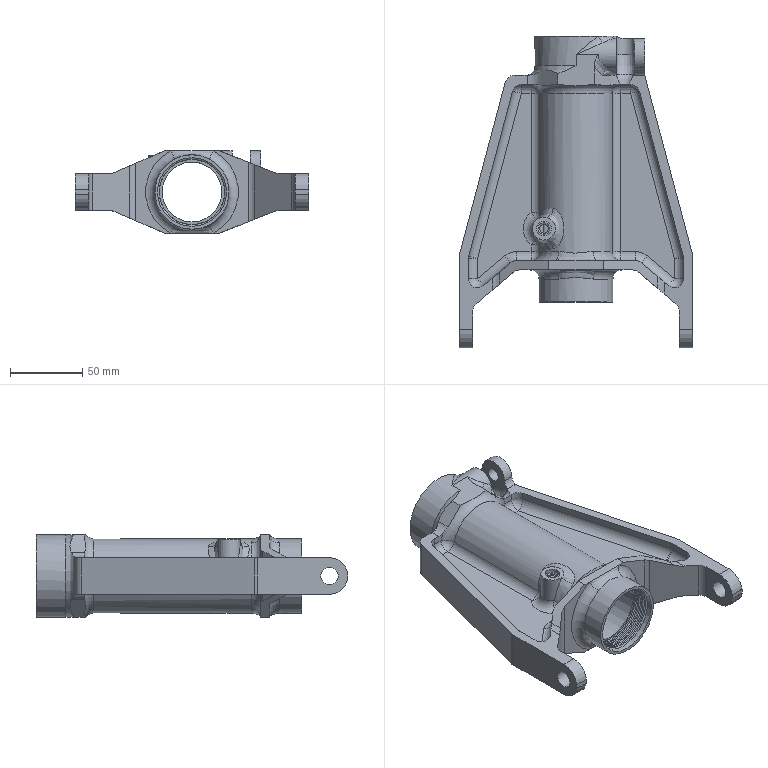Part | NX | features MG0330 trunion parts 24(trunion group) 2 | 1 solid | 262 faces | volume 256583 mm3 | cylinder 92 | plane 78 | cone 34 | sphere 25 | torus 18 | spline 15 | commonest cylinder face diameters 12.7 x51 25.4 x12 9.525 x8 51.598 x3 11.913 x2 22.225 x2